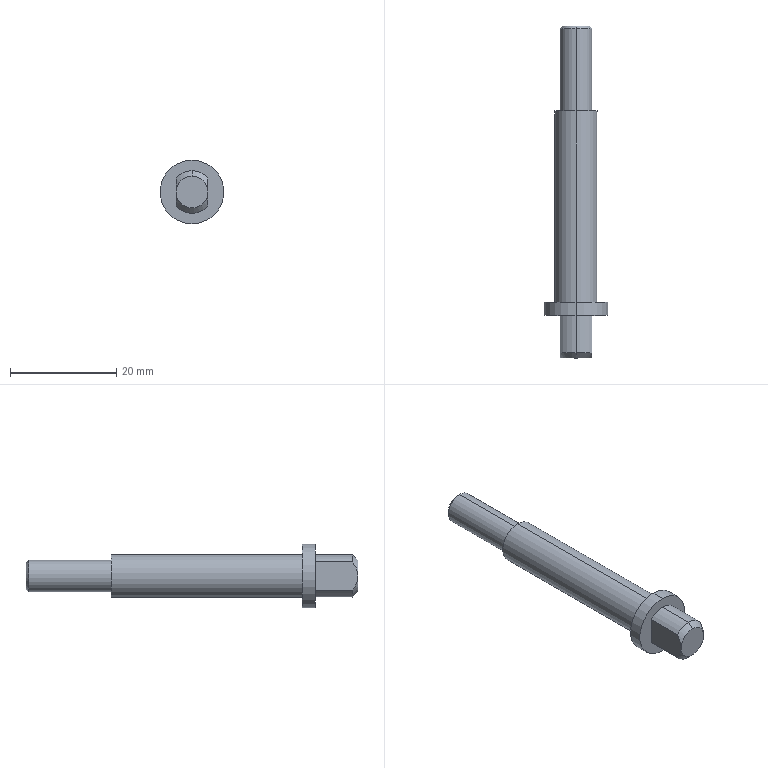Part | STEP file | 18 | 1 solid | 21 faces | box 12 x 62.5 x 12 mm | volume 2879 mm3 | cylinder 9 | plane 7 | cone 5 | commonest cylinder face diameters 8 x5 6 x2 12 x2